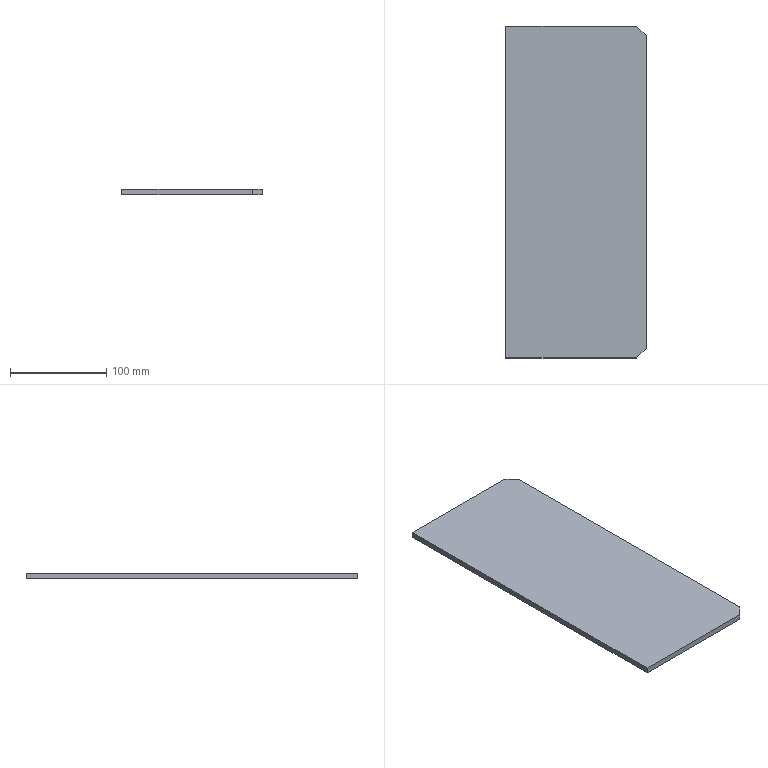Part | STEP file | 03-Rib plate 3 | 1 solid | 8 faces | box 146 x 345 x 6 mm | volume 301620 mm3 | plane 8
STEP:
#1=CARTESIAN_POINT('',(0.,0.,0.));
#2=DIRECTION('',(0.,0.,1.));
#3=DIRECTION('',(1.,0.,0.));
#4=AXIS2_PLACEMENT_3D('',#1,#2,#3);
#5=CARTESIAN_POINT('',(0.,0.,0.));
#6=VERTEX_POINT('',#5);
#7=CARTESIAN_POINT('',(0.,-345.,0.));
#8=VERTEX_POINT('',#7);
#9=CARTESIAN_POINT('',(0.,0.,0.));
#10=DIRECTION('',(0.,-1.,0.));
#11=VECTOR('',#10,1.);
#12=LINE('',#9,#11);
#13=CARTESIAN_POINT('',(0.,0.,6.));
#14=DIRECTION('',(1.,0.,0.));
#15=DIRECTION('',(0.,1.,0.));
#16=AXIS2_PLACEMENT_3D('',#13,#14,#15);
#17=PLANE('',#16);
#18=CARTESIAN_POINT('',(0.,-6.));
#19=DIRECTION('',(-1.,0.));
#20=VECTOR('',#19,1.);
#21=LINE('',#18,#20);
#22=(GEOMETRIC_REPRESENTATION_CONTEXT(2)PARAMETRIC_REPRESENTATION_CONTEXT()REPRESENTATION_CONTEXT('',''));
#23=DEFINITIONAL_REPRESENTATION('',(#21),#22);
#24=PCURVE('',#17,#23);
#25=CARTESIAN_POINT('',(0.,0.,0.));
#26=DIRECTION('',(0.,0.,1.));
#27=DIRECTION('',(1.,0.,0.));
#28=AXIS2_PLACEMENT_3D('',#25,#26,#27);
#29=PLANE('',#28);
#30=CARTESIAN_POINT('',(0.,0.));
#31=DIRECTION('',(0.,-1.));
#32=VECTOR('',#31,1.);
#33=LINE('',#30,#32);
#34=(GEOMETRIC_REPRESENTATION_CONTEXT(2)PARAMETRIC_REPRESENTATION_CONTEXT()REPRESENTATION_CONTEXT('',''));
#35=DEFINITIONAL_REPRESENTATION('',(#33),#34);
#36=PCURVE('',#29,#35);
#37=SURFACE_CURVE('',#12,(#24,#36),.PCURVE_S1.);
#38=EDGE_CURVE('',#6,#8,#37,.T.);
#39=ORIENTED_EDGE('',*,*,#38,.T.);
#40=CARTESIAN_POINT('',(0.,-345.,6.));
#41=VERTEX_POINT('',#40);
#42=CARTESIAN_POINT('',(0.,-345.,6.));
#43=DIRECTION('',(0.,0.,-1.));
#44=VECTOR('',#43,1.);
#45=LINE('',#42,#44);
#46=CARTESIAN_POINT('',(-345.,0.));
#47=DIRECTION('',(0.,-1.));
#48=VECTOR('',#47,1.);
#49=LINE('',#46,#48);
#50=(GEOMETRIC_REPRESENTATION_CONTEXT(2)PARAMETRIC_REPRESENTATION_CONTEXT()REPRESENTATION_CONTEXT('',''));
#51=DEFINITIONAL_REPRESENTATION('',(#49),#50);
#52=PCURVE('',#17,#51);
#53=CARTESIAN_POINT('',(0.,-345.,6.));
#54=DIRECTION('',(0.,1.,0.));
#55=DIRECTION('',(0.,0.,1.));
#56=AXIS2_PLACEMENT_3D('',#53,#54,#55);
#57=PLANE('',#56);
#58=CARTESIAN_POINT('',(0.,0.));
#59=DIRECTION('',(-1.,0.));
#60=VECTOR('',#59,1.);
#61=LINE('',#58,#60);
#62=(GEOMETRIC_REPRESENTATION_CONTEXT(2)PARAMETRIC_REPRESENTATION_CONTEXT()REPRESENTATION_CONTEXT('',''));
#63=DEFINITIONAL_REPRESENTATION('',(#61),#62);
#64=PCURVE('',#57,#63);
#65=SURFACE_CURVE('',#45,(#52,#64),.PCURVE_S1.);
#66=EDGE_CURVE('',#41,#8,#65,.T.);
#67=ORIENTED_EDGE('',*,*,#66,.F.);
#68=CARTESIAN_POINT('',(0.,0.,6.));
#69=VERTEX_POINT('',#68);
#70=CARTESIAN_POINT('',(0.,0.,6.));
#71=DIRECTION('',(0.,-1.,0.));
#72=VECTOR('',#71,1.);
#73=LINE('',#70,#72);
#74=CARTESIAN_POINT('',(0.,0.));
#75=DIRECTION('',(-1.,0.));
#76=VECTOR('',#75,1.);
#77=LINE('',#74,#76);
#78=(GEOMETRIC_REPRESENTATION_CONTEXT(2)PARAMETRIC_REPRESENTATION_CONTEXT()REPRESENTATION_CONTEXT('',''));
#79=DEFINITIONAL_REPRESENTATION('',(#77),#78);
#80=PCURVE('',#17,#79);
#81=CARTESIAN_POINT('',(0.,0.,6.));
#82=DIRECTION('',(0.,0.,1.));
#83=DIRECTION('',(1.,0.,0.));
#84=AXIS2_PLACEMENT_3D('',#81,#82,#83);
#85=PLANE('',#84);
#86=CARTESIAN_POINT('',(0.,0.));
#87=DIRECTION('',(0.,-1.));
#88=VECTOR('',#87,1.);
#89=LINE('',#86,#88);
#90=(GEOMETRIC_REPRESENTATION_CONTEXT(2)PARAMETRIC_REPRESENTATION_CONTEXT()REPRESENTATION_CONTEXT('',''));
#91=DEFINITIONAL_REPRESENTATION('',(#89),#90);
#92=PCURVE('',#85,#91);
#93=SURFACE_CURVE('',#73,(#80,#92),.PCURVE_S1.);
#94=EDGE_CURVE('',#69,#41,#93,.T.);
#95=ORIENTED_EDGE('',*,*,#94,.F.);
#96=CARTESIAN_POINT('',(0.,0.,6.));
#97=DIRECTION('',(0.,0.,-1.));
#98=VECTOR('',#97,1.);
#99=LINE('',#96,#98);
#100=CARTESIAN_POINT('',(0.,0.));
#101=DIRECTION('',(0.,-1.));
#102=VECTOR('',#101,1.);
#103=LINE('',#100,#102);
#104=(GEOMETRIC_REPRESENTATION_CONTEXT(2)PARAMETRIC_REPRESENTATION_CONTEXT()REPRESENTATION_CONTEXT('',''));
#105=DEFINITIONAL_REPRESENTATION('',(#103),#104);
#106=PCURVE('',#17,#105);
#107=CARTESIAN_POINT('',(0.,0.,6.));
#108=DIRECTION('',(0.,-1.,0.));
#109=DIRECTION('',(0.,0.,-1.));
#110=AXIS2_PLACEMENT_3D('',#107,#108,#109);
#111=PLANE('',#110);
#112=CARTESIAN_POINT('',(0.,0.));
#113=DIRECTION('',(1.,0.));
#114=VECTOR('',#113,1.);
#115=LINE('',#112,#114);
#116=(GEOMETRIC_REPRESENTATION_CONTEXT(2)PARAMETRIC_REPRESENTATION_CONTEXT()REPRESENTATION_CONTEXT('',''));
#117=DEFINITIONAL_REPRESENTATION('',(#115),#116);
#118=PCURVE('',#111,#117);
#119=SURFACE_CURVE('',#99,(#106,#118),.PCURVE_S1.);
#120=EDGE_CURVE('',#69,#6,#119,.T.);
#121=ORIENTED_EDGE('',*,*,#120,.T.);
#122=EDGE_LOOP('',(#39,#67,#95,#121));
#123=FACE_BOUND('',#122,.T.);
#124=ADVANCED_FACE('',(#123),#17,.F.);
#125=CARTESIAN_POINT('',(136.,-345.,0.));
#126=VERTEX_POINT('',#125);
#127=CARTESIAN_POINT('',(0.,-345.,0.));
#128=DIRECTION('',(1.,0.,0.));
#129=VECTOR('',#128,1.);
#130=LINE('',#127,#129);
#131=CARTESIAN_POINT('',(-6.,0.));
#132=DIRECTION('',(0.,1.));
#133=VECTOR('',#132,1.);
#134=LINE('',#131,#133);
#135=(GEOMETRIC_REPRESENTATION_CONTEXT(2)PARAMETRIC_REPRESENTATION_CONTEXT()REPRESENTATION_CONTEXT('',''));
#136=DEFINITIONAL_REPRESENTATION('',(#134),#135);
#137=PCURVE('',#57,#136);
#138=CARTESIAN_POINT('',(0.,-345.));
#139=DIRECTION('',(1.,0.));
#140=VECTOR('',#139,1.);
#141=LINE('',#138,#140);
#142=(GEOMETRIC_REPRESENTATION_CONTEXT(2)PARAMETRIC_REPRESENTATION_CONTEXT()REPRESENTATION_CONTEXT('',''));
#143=DEFINITIONAL_REPRESENTATION('',(#141),#142);
#144=PCURVE('',#29,#143);
#145=SURFACE_CURVE('',#130,(#137,#144),.PCURVE_S1.);
#146=EDGE_CURVE('',#8,#126,#145,.T.);
#147=ORIENTED_EDGE('',*,*,#146,.T.);
#148=CARTESIAN_POINT('',(136.,-345.,6.));
#149=VERTEX_POINT('',#148);
#150=CARTESIAN_POINT('',(136.,-345.,6.));
#151=DIRECTION('',(0.,0.,-1.));
#152=VECTOR('',#151,1.);
#153=LINE('',#150,#152);
#154=CARTESIAN_POINT('',(0.,136.));
#155=DIRECTION('',(-1.,0.));
#156=VECTOR('',#155,1.);
#157=LINE('',#154,#156);
#158=(GEOMETRIC_REPRESENTATION_CONTEXT(2)PARAMETRIC_REPRESENTATION_CONTEXT()REPRESENTATION_CONTEXT('',''));
#159=DEFINITIONAL_REPRESENTATION('',(#157),#158);
#160=PCURVE('',#57,#159);
#161=CARTESIAN_POINT('',(146.,-335.,6.));
#162=DIRECTION('',(-0.7071,0.7071,0.));
#163=DIRECTION('',(-0.7071,-0.7071,0.));
#164=AXIS2_PLACEMENT_3D('',#161,#162,#163);
#165=PLANE('',#164);
#166=CARTESIAN_POINT('',(14.142,0.));
#167=DIRECTION('',(0.,-1.));
#168=VECTOR('',#167,1.);
#169=LINE('',#166,#168);
#170=(GEOMETRIC_REPRESENTATION_CONTEXT(2)PARAMETRIC_REPRESENTATION_CONTEXT()REPRESENTATION_CONTEXT('',''));
#171=DEFINITIONAL_REPRESENTATION('',(#169),#170);
#172=PCURVE('',#165,#171);
#173=SURFACE_CURVE('',#153,(#160,#172),.PCURVE_S1.);
#174=EDGE_CURVE('',#149,#126,#173,.T.);
#175=ORIENTED_EDGE('',*,*,#174,.F.);
#176=CARTESIAN_POINT('',(0.,-345.,6.));
#177=DIRECTION('',(1.,0.,0.));
#178=VECTOR('',#177,1.);
#179=LINE('',#176,#178);
#180=CARTESIAN_POINT('',(0.,0.));
#181=DIRECTION('',(0.,1.));
#182=VECTOR('',#181,1.);
#183=LINE('',#180,#182);
#184=(GEOMETRIC_REPRESENTATION_CONTEXT(2)PARAMETRIC_REPRESENTATION_CONTEXT()REPRESENTATION_CONTEXT('',''));
#185=DEFINITIONAL_REPRESENTATION('',(#183),#184);
#186=PCURVE('',#57,#185);
#187=CARTESIAN_POINT('',(0.,-345.));
#188=DIRECTION('',(1.,0.));
#189=VECTOR('',#188,1.);
#190=LINE('',#187,#189);
#191=(GEOMETRIC_REPRESENTATION_CONTEXT(2)PARAMETRIC_REPRESENTATION_CONTEXT()REPRESENTATION_CONTEXT('',''));
#192=DEFINITIONAL_REPRESENTATION('',(#190),#191);
#193=PCURVE('',#85,#192);
#194=SURFACE_CURVE('',#179,(#186,#193),.PCURVE_S1.);
#195=EDGE_CURVE('',#41,#149,#194,.T.);
#196=ORIENTED_EDGE('',*,*,#195,.F.);
#197=ORIENTED_EDGE('',*,*,#66,.T.);
#198=EDGE_LOOP('',(#147,#175,#196,#197));
#199=FACE_BOUND('',#198,.T.);
#200=ADVANCED_FACE('',(#199),#57,.F.);
#201=CARTESIAN_POINT('',(146.,-335.,0.));
#202=VERTEX_POINT('',#201);
#203=CARTESIAN_POINT('',(146.,-335.,0.));
#204=DIRECTION('',(0.7071,0.7071,0.));
#205=VECTOR('',#204,1.);
#206=LINE('',#203,#205);
#207=CARTESIAN_POINT('',(0.,-6.));
#208=DIRECTION('',(-1.,0.));
#209=VECTOR('',#208,1.);
#210=LINE('',#207,#209);
#211=(GEOMETRIC_REPRESENTATION_CONTEXT(2)PARAMETRIC_REPRESENTATION_CONTEXT()REPRESENTATION_CONTEXT('',''));
#212=DEFINITIONAL_REPRESENTATION('',(#210),#211);
#213=PCURVE('',#165,#212);
#214=CARTESIAN_POINT('',(146.,-335.));
#215=DIRECTION('',(0.7071,0.7071));
#216=VECTOR('',#215,1.);
#217=LINE('',#214,#216);
#218=(GEOMETRIC_REPRESENTATION_CONTEXT(2)PARAMETRIC_REPRESENTATION_CONTEXT()REPRESENTATION_CONTEXT('',''));
#219=DEFINITIONAL_REPRESENTATION('',(#217),#218);
#220=PCURVE('',#29,#219);
#221=SURFACE_CURVE('',#206,(#213,#220),.PCURVE_S1.);
#222=EDGE_CURVE('',#126,#202,#221,.T.);
#223=ORIENTED_EDGE('',*,*,#222,.T.);
#224=CARTESIAN_POINT('',(146.,-335.,6.));
#225=VERTEX_POINT('',#224);
#226=CARTESIAN_POINT('',(146.,-335.,6.));
#227=DIRECTION('',(0.,0.,-1.));
#228=VECTOR('',#227,1.);
#229=LINE('',#226,#228);
#230=CARTESIAN_POINT('',(0.,0.));
#231=DIRECTION('',(0.,-1.));
#232=VECTOR('',#231,1.);
#233=LINE('',#230,#232);
#234=(GEOMETRIC_REPRESENTATION_CONTEXT(2)PARAMETRIC_REPRESENTATION_CONTEXT()REPRESENTATION_CONTEXT('',''));
#235=DEFINITIONAL_REPRESENTATION('',(#233),#234);
#236=PCURVE('',#165,#235);
#237=CARTESIAN_POINT('',(146.,-10.,6.));
#238=DIRECTION('',(-1.,0.,0.));
#239=DIRECTION('',(0.,-1.,0.));
#240=AXIS2_PLACEMENT_3D('',#237,#238,#239);
#241=PLANE('',#240);
#242=CARTESIAN_POINT('',(325.,0.));
#243=DIRECTION('',(0.,-1.));
#244=VECTOR('',#243,1.);
#245=LINE('',#242,#244);
#246=(GEOMETRIC_REPRESENTATION_CONTEXT(2)PARAMETRIC_REPRESENTATION_CONTEXT()REPRESENTATION_CONTEXT('',''));
#247=DEFINITIONAL_REPRESENTATION('',(#245),#246);
#248=PCURVE('',#241,#247);
#249=SURFACE_CURVE('',#229,(#236,#248),.PCURVE_S1.);
#250=EDGE_CURVE('',#225,#202,#249,.T.);
#251=ORIENTED_EDGE('',*,*,#250,.F.);
#252=CARTESIAN_POINT('',(146.,-335.,6.));
#253=DIRECTION('',(0.7071,0.7071,0.));
#254=VECTOR('',#253,1.);
#255=LINE('',#252,#254);
#256=CARTESIAN_POINT('',(0.,0.));
#257=DIRECTION('',(-1.,0.));
#258=VECTOR('',#257,1.);
#259=LINE('',#256,#258);
#260=(GEOMETRIC_REPRESENTATION_CONTEXT(2)PARAMETRIC_REPRESENTATION_CONTEXT()REPRESENTATION_CONTEXT('',''));
#261=DEFINITIONAL_REPRESENTATION('',(#259),#260);
#262=PCURVE('',#165,#261);
#263=CARTESIAN_POINT('',(146.,-335.));
#264=DIRECTION('',(0.7071,0.7071));
#265=VECTOR('',#264,1.);
#266=LINE('',#263,#265);
#267=(GEOMETRIC_REPRESENTATION_CONTEXT(2)PARAMETRIC_REPRESENTATION_CONTEXT()REPRESENTATION_CONTEXT('',''));
#268=DEFINITIONAL_REPRESENTATION('',(#266),#267);
#269=PCURVE('',#85,#268);
#270=SURFACE_CURVE('',#255,(#262,#269),.PCURVE_S1.);
#271=EDGE_CURVE('',#149,#225,#270,.T.);
#272=ORIENTED_EDGE('',*,*,#271,.F.);
#273=ORIENTED_EDGE('',*,*,#174,.T.);
#274=EDGE_LOOP('',(#223,#251,#272,#273));
#275=FACE_BOUND('',#274,.T.);
#276=ADVANCED_FACE('',(#275),#165,.F.);
#277=CARTESIAN_POINT('',(146.,-10.,0.));
#278=VERTEX_POINT('',#277);
#279=CARTESIAN_POINT('',(146.,-10.,0.));
#280=DIRECTION('',(0.,1.,0.));
#281=VECTOR('',#280,1.);
#282=LINE('',#279,#281);
#283=CARTESIAN_POINT('',(0.,-6.));
#284=DIRECTION('',(-1.,0.));
#285=VECTOR('',#284,1.);
#286=LINE('',#283,#285);
#287=(GEOMETRIC_REPRESENTATION_CONTEXT(2)PARAMETRIC_REPRESENTATION_CONTEXT()REPRESENTATION_CONTEXT('',''));
#288=DEFINITIONAL_REPRESENTATION('',(#286),#287);
#289=PCURVE('',#241,#288);
#290=CARTESIAN_POINT('',(146.,-10.));
#291=DIRECTION('',(0.,1.));
#292=VECTOR('',#291,1.);
#293=LINE('',#290,#292);
#294=(GEOMETRIC_REPRESENTATION_CONTEXT(2)PARAMETRIC_REPRESENTATION_CONTEXT()REPRESENTATION_CONTEXT('',''));
#295=DEFINITIONAL_REPRESENTATION('',(#293),#294);
#296=PCURVE('',#29,#295);
#297=SURFACE_CURVE('',#282,(#289,#296),.PCURVE_S1.);
#298=EDGE_CURVE('',#202,#278,#297,.T.);
#299=ORIENTED_EDGE('',*,*,#298,.T.);
#300=CARTESIAN_POINT('',(146.,-10.,6.));
#301=VERTEX_POINT('',#300);
#302=CARTESIAN_POINT('',(146.,-10.,6.));
#303=DIRECTION('',(0.,0.,-1.));
#304=VECTOR('',#303,1.);
#305=LINE('',#302,#304);
#306=CARTESIAN_POINT('',(0.,0.));
#307=DIRECTION('',(0.,-1.));
#308=VECTOR('',#307,1.);
#309=LINE('',#306,#308);
#310=(GEOMETRIC_REPRESENTATION_CONTEXT(2)PARAMETRIC_REPRESENTATION_CONTEXT()REPRESENTATION_CONTEXT('',''));
#311=DEFINITIONAL_REPRESENTATION('',(#309),#310);
#312=PCURVE('',#241,#311);
#313=CARTESIAN_POINT('',(136.,0.,6.));
#314=DIRECTION('',(-0.7071,-0.7071,0.));
#315=DIRECTION('',(0.7071,-0.7071,0.));
#316=AXIS2_PLACEMENT_3D('',#313,#314,#315);
#317=PLANE('',#316);
#318=CARTESIAN_POINT('',(14.142,0.));
#319=DIRECTION('',(0.,-1.));
#320=VECTOR('',#319,1.);
#321=LINE('',#318,#320);
#322=(GEOMETRIC_REPRESENTATION_CONTEXT(2)PARAMETRIC_REPRESENTATION_CONTEXT()REPRESENTATION_CONTEXT('',''));
#323=DEFINITIONAL_REPRESENTATION('',(#321),#322);
#324=PCURVE('',#317,#323);
#325=SURFACE_CURVE('',#305,(#312,#324),.PCURVE_S1.);
#326=EDGE_CURVE('',#301,#278,#325,.T.);
#327=ORIENTED_EDGE('',*,*,#326,.F.);
#328=CARTESIAN_POINT('',(146.,-10.,6.));
#329=DIRECTION('',(0.,1.,0.));
#330=VECTOR('',#329,1.);
#331=LINE('',#328,#330);
#332=CARTESIAN_POINT('',(0.,0.));
#333=DIRECTION('',(-1.,0.));
#334=VECTOR('',#333,1.);
#335=LINE('',#332,#334);
#336=(GEOMETRIC_REPRESENTATION_CONTEXT(2)PARAMETRIC_REPRESENTATION_CONTEXT()REPRESENTATION_CONTEXT('',''));
#337=DEFINITIONAL_REPRESENTATION('',(#335),#336);
#338=PCURVE('',#241,#337);
#339=CARTESIAN_POINT('',(146.,-10.));
#340=DIRECTION('',(0.,1.));
#341=VECTOR('',#340,1.);
#342=LINE('',#339,#341);
#343=(GEOMETRIC_REPRESENTATION_CONTEXT(2)PARAMETRIC_REPRESENTATION_CONTEXT()REPRESENTATION_CONTEXT('',''));
#344=DEFINITIONAL_REPRESENTATION('',(#342),#343);
#345=PCURVE('',#85,#344);
#346=SURFACE_CURVE('',#331,(#338,#345),.PCURVE_S1.);
#347=EDGE_CURVE('',#225,#301,#346,.T.);
#348=ORIENTED_EDGE('',*,*,#347,.F.);
#349=ORIENTED_EDGE('',*,*,#250,.T.);
#350=EDGE_LOOP('',(#299,#327,#348,#349));
#351=FACE_BOUND('',#350,.T.);
#352=ADVANCED_FACE('',(#351),#241,.F.);
#353=CARTESIAN_POINT('',(136.,0.,0.));
#354=VERTEX_POINT('',#353);
#355=CARTESIAN_POINT('',(136.,0.,0.));
#356=DIRECTION('',(-0.7071,0.7071,0.));
#357=VECTOR('',#356,1.);
#358=LINE('',#355,#357);
#359=CARTESIAN_POINT('',(0.,-6.));
#360=DIRECTION('',(-1.,0.));
#361=VECTOR('',#360,1.);
#362=LINE('',#359,#361);
#363=(GEOMETRIC_REPRESENTATION_CONTEXT(2)PARAMETRIC_REPRESENTATION_CONTEXT()REPRESENTATION_CONTEXT('',''));
#364=DEFINITIONAL_REPRESENTATION('',(#362),#363);
#365=PCURVE('',#317,#364);
#366=CARTESIAN_POINT('',(136.,0.));
#367=DIRECTION('',(-0.7071,0.7071));
#368=VECTOR('',#367,1.);
#369=LINE('',#366,#368);
#370=(GEOMETRIC_REPRESENTATION_CONTEXT(2)PARAMETRIC_REPRESENTATION_CONTEXT()REPRESENTATION_CONTEXT('',''));
#371=DEFINITIONAL_REPRESENTATION('',(#369),#370);
#372=PCURVE('',#29,#371);
#373=SURFACE_CURVE('',#358,(#365,#372),.PCURVE_S1.);
#374=EDGE_CURVE('',#278,#354,#373,.T.);
#375=ORIENTED_EDGE('',*,*,#374,.T.);
#376=CARTESIAN_POINT('',(136.,0.,6.));
#377=VERTEX_POINT('',#376);
#378=CARTESIAN_POINT('',(136.,0.,6.));
#379=DIRECTION('',(0.,0.,-1.));
#380=VECTOR('',#379,1.);
#381=LINE('',#378,#380);
#382=CARTESIAN_POINT('',(0.,0.));
#383=DIRECTION('',(0.,-1.));
#384=VECTOR('',#383,1.);
#385=LINE('',#382,#384);
#386=(GEOMETRIC_REPRESENTATION_CONTEXT(2)PARAMETRIC_REPRESENTATION_CONTEXT()REPRESENTATION_CONTEXT('',''));
#387=DEFINITIONAL_REPRESENTATION('',(#385),#386);
#388=PCURVE('',#317,#387);
#389=CARTESIAN_POINT('',(0.,136.));
#390=DIRECTION('',(1.,0.));
#391=VECTOR('',#390,1.);
#392=LINE('',#389,#391);
#393=(GEOMETRIC_REPRESENTATION_CONTEXT(2)PARAMETRIC_REPRESENTATION_CONTEXT()REPRESENTATION_CONTEXT('',''));
#394=DEFINITIONAL_REPRESENTATION('',(#392),#393);
#395=PCURVE('',#111,#394);
#396=SURFACE_CURVE('',#381,(#388,#395),.PCURVE_S1.);
#397=EDGE_CURVE('',#377,#354,#396,.T.);
#398=ORIENTED_EDGE('',*,*,#397,.F.);
#399=CARTESIAN_POINT('',(136.,0.,6.));
#400=DIRECTION('',(-0.7071,0.7071,0.));
#401=VECTOR('',#400,1.);
#402=LINE('',#399,#401);
#403=CARTESIAN_POINT('',(0.,0.));
#404=DIRECTION('',(-1.,0.));
#405=VECTOR('',#404,1.);
#406=LINE('',#403,#405);
#407=(GEOMETRIC_REPRESENTATION_CONTEXT(2)PARAMETRIC_REPRESENTATION_CONTEXT()REPRESENTATION_CONTEXT('',''));
#408=DEFINITIONAL_REPRESENTATION('',(#406),#407);
#409=PCURVE('',#317,#408);
#410=CARTESIAN_POINT('',(136.,0.));
#411=DIRECTION('',(-0.7071,0.7071));
#412=VECTOR('',#411,1.);
#413=LINE('',#410,#412);
#414=(GEOMETRIC_REPRESENTATION_CONTEXT(2)PARAMETRIC_REPRESENTATION_CONTEXT()REPRESENTATION_CONTEXT('',''));
#415=DEFINITIONAL_REPRESENTATION('',(#413),#414);
#416=PCURVE('',#85,#415);
#417=SURFACE_CURVE('',#402,(#409,#416),.PCURVE_S1.);
#418=EDGE_CURVE('',#301,#377,#417,.T.);
#419=ORIENTED_EDGE('',*,*,#418,.F.);
#420=ORIENTED_EDGE('',*,*,#326,.T.);
#421=EDGE_LOOP('',(#375,#398,#419,#420));
#422=FACE_BOUND('',#421,.T.);
#423=ADVANCED_FACE('',(#422),#317,.F.);
#424=CARTESIAN_POINT('',(0.,0.,0.));
#425=DIRECTION('',(-1.,0.,0.));
#426=VECTOR('',#425,1.);
#427=LINE('',#424,#426);
#428=CARTESIAN_POINT('',(6.,0.));
#429=DIRECTION('',(0.,-1.));
#430=VECTOR('',#429,1.);
#431=LINE('',#428,#430);
#432=(GEOMETRIC_REPRESENTATION_CONTEXT(2)PARAMETRIC_REPRESENTATION_CONTEXT()REPRESENTATION_CONTEXT('',''));
#433=DEFINITIONAL_REPRESENTATION('',(#431),#432);
#434=PCURVE('',#111,#433);
#435=CARTESIAN_POINT('',(0.,0.));
#436=DIRECTION('',(-1.,0.));
#437=VECTOR('',#436,1.);
#438=LINE('',#435,#437);
#439=(GEOMETRIC_REPRESENTATION_CONTEXT(2)PARAMETRIC_REPRESENTATION_CONTEXT()REPRESENTATION_CONTEXT('',''));
#440=DEFINITIONAL_REPRESENTATION('',(#438),#439);
#441=PCURVE('',#29,#440);
#442=SURFACE_CURVE('',#427,(#434,#441),.PCURVE_S1.);
#443=EDGE_CURVE('',#354,#6,#442,.T.);
#444=ORIENTED_EDGE('',*,*,#443,.T.);
#445=ORIENTED_EDGE('',*,*,#120,.F.);
#446=CARTESIAN_POINT('',(0.,0.,6.));
#447=DIRECTION('',(-1.,0.,0.));
#448=VECTOR('',#447,1.);
#449=LINE('',#446,#448);
#450=CARTESIAN_POINT('',(0.,0.));
#451=DIRECTION('',(0.,-1.));
#452=VECTOR('',#451,1.);
#453=LINE('',#450,#452);
#454=(GEOMETRIC_REPRESENTATION_CONTEXT(2)PARAMETRIC_REPRESENTATION_CONTEXT()REPRESENTATION_CONTEXT('',''));
#455=DEFINITIONAL_REPRESENTATION('',(#453),#454);
#456=PCURVE('',#111,#455);
#457=CARTESIAN_POINT('',(0.,0.));
#458=DIRECTION('',(-1.,0.));
#459=VECTOR('',#458,1.);
#460=LINE('',#457,#459);
#461=(GEOMETRIC_REPRESENTATION_CONTEXT(2)PARAMETRIC_REPRESENTATION_CONTEXT()REPRESENTATION_CONTEXT('',''));
#462=DEFINITIONAL_REPRESENTATION('',(#460),#461);
#463=PCURVE('',#85,#462);
#464=SURFACE_CURVE('',#449,(#456,#463),.PCURVE_S1.);
#465=EDGE_CURVE('',#377,#69,#464,.T.);
#466=ORIENTED_EDGE('',*,*,#465,.F.);
#467=ORIENTED_EDGE('',*,*,#397,.T.);
#468=EDGE_LOOP('',(#444,#445,#466,#467));
#469=FACE_BOUND('',#468,.T.);
#470=ADVANCED_FACE('',(#469),#111,.F.);
#471=ORIENTED_EDGE('',*,*,#94,.T.);
#472=ORIENTED_EDGE('',*,*,#195,.T.);
#473=ORIENTED_EDGE('',*,*,#271,.T.);
#474=ORIENTED_EDGE('',*,*,#347,.T.);
#475=ORIENTED_EDGE('',*,*,#418,.T.);
#476=ORIENTED_EDGE('',*,*,#465,.T.);
#477=EDGE_LOOP('',(#471,#472,#473,#474,#475,#476));
#478=FACE_BOUND('',#477,.T.);
#479=ADVANCED_FACE('',(#478),#85,.T.);
#480=ORIENTED_EDGE('',*,*,#38,.F.);
#481=ORIENTED_EDGE('',*,*,#443,.F.);
#482=ORIENTED_EDGE('',*,*,#374,.F.);
#483=ORIENTED_EDGE('',*,*,#298,.F.);
#484=ORIENTED_EDGE('',*,*,#222,.F.);
#485=ORIENTED_EDGE('',*,*,#146,.F.);
#486=EDGE_LOOP('',(#480,#481,#482,#483,#484,#485));
#487=FACE_BOUND('',#486,.T.);
#488=ADVANCED_FACE('',(#487),#29,.F.);
#489=CLOSED_SHELL('',(#124,#200,#276,#352,#423,#470,#479,#488));
#490=MANIFOLD_SOLID_BREP('',#489);
#491=(LENGTH_UNIT()NAMED_UNIT(*)SI_UNIT(.MILLI.,.METRE.));
#492=UNCERTAINTY_MEASURE_WITH_UNIT(LENGTH_MEASURE(0.0000001),#491,'','');
#493=(NAMED_UNIT(*)PLANE_ANGLE_UNIT()SI_UNIT($,.RADIAN.));
#494=(NAMED_UNIT(*)SI_UNIT($,.STERADIAN.)SOLID_ANGLE_UNIT());
#495=(GEOMETRIC_REPRESENTATION_CONTEXT(3)GLOBAL_UNCERTAINTY_ASSIGNED_CONTEXT((#492))GLOBAL_UNIT_ASSIGNED_CONTEXT((#491,#493,#494))REPRESENTATION_CONTEXT('',''));
#496=ADVANCED_BREP_SHAPE_REPRESENTATION('',(#4,#490),#495);